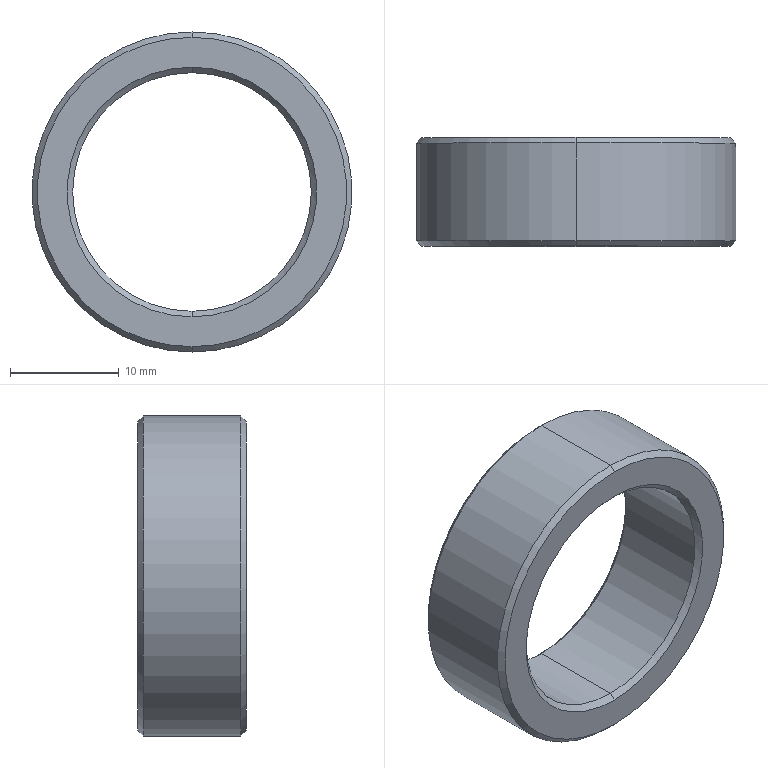Part | STEP file | Cuon T phu H01_3 | 1 solid | 14 faces | box 29.5 x 10 x 29.5 mm | volume 2993 mm3 | cone 8 | cylinder 4 | plane 2 | commonest cylinder face diameters 22 x2 29.5 x2
STEP:
#1=CARTESIAN_POINT('',(0.,0.,0.));
#2=DIRECTION('',(0.,0.,1.));
#3=DIRECTION('',(1.,0.,0.));
#4=AXIS2_PLACEMENT_3D('',#1,#2,#3);
#5=CARTESIAN_POINT('',(0.,9.5,11.));
#6=VERTEX_POINT('',#5);
#7=CARTESIAN_POINT('',(0.,10.,11.5));
#8=VERTEX_POINT('',#7);
#9=CARTESIAN_POINT('',(0.,9.5,11.));
#10=DIRECTION('',(0.,0.7071,0.7071));
#11=VECTOR('',#10,1.);
#12=LINE('',#9,#11);
#13=CARTESIAN_POINT('',(0.,9.5,0.));
#14=DIRECTION('',(0.,1.,0.));
#15=DIRECTION('',(0.,0.,1.));
#16=AXIS2_PLACEMENT_3D('',#13,#14,#15);
#17=CONICAL_SURFACE('',#16,11.,0.7854);
#18=CARTESIAN_POINT('',(6.283,0.));
#19=DIRECTION('',(0.,1.));
#20=VECTOR('',#19,1.);
#21=LINE('',#18,#20);
#22=(GEOMETRIC_REPRESENTATION_CONTEXT(2)PARAMETRIC_REPRESENTATION_CONTEXT()REPRESENTATION_CONTEXT('',''));
#23=DEFINITIONAL_REPRESENTATION('',(#21),#22);
#24=PCURVE('',#17,#23);
#25=CARTESIAN_POINT('',(0.,9.5,0.));
#26=DIRECTION('',(0.,1.,0.));
#27=DIRECTION('',(0.,0.,1.));
#28=AXIS2_PLACEMENT_3D('',#25,#26,#27);
#29=CONICAL_SURFACE('',#28,11.,0.7854);
#30=CARTESIAN_POINT('',(0.,0.));
#31=DIRECTION('',(0.,1.));
#32=VECTOR('',#31,1.);
#33=LINE('',#30,#32);
#34=(GEOMETRIC_REPRESENTATION_CONTEXT(2)PARAMETRIC_REPRESENTATION_CONTEXT()REPRESENTATION_CONTEXT('',''));
#35=DEFINITIONAL_REPRESENTATION('',(#33),#34);
#36=PCURVE('',#29,#35);
#37=SURFACE_CURVE('',#12,(#24,#36),.PCURVE_S1.);
#38=EDGE_CURVE('',#6,#8,#37,.T.);
#39=ORIENTED_EDGE('',*,*,#38,.T.);
#40=CARTESIAN_POINT('',(0.,10.,-11.5));
#41=VERTEX_POINT('',#40);
#42=CARTESIAN_POINT('',(0.,10.,0.));
#43=DIRECTION('',(0.,-1.,0.));
#44=DIRECTION('',(0.,0.,1.));
#45=AXIS2_PLACEMENT_3D('',#42,#43,#44);
#46=CIRCLE('',#45,11.5);
#47=CARTESIAN_POINT('',(6.283,0.5));
#48=DIRECTION('',(-1.,0.));
#49=VECTOR('',#48,1.);
#50=LINE('',#47,#49);
#51=(GEOMETRIC_REPRESENTATION_CONTEXT(2)PARAMETRIC_REPRESENTATION_CONTEXT()REPRESENTATION_CONTEXT('',''));
#52=DEFINITIONAL_REPRESENTATION('',(#50),#51);
#53=PCURVE('',#17,#52);
#54=CARTESIAN_POINT('',(0.,10.,0.));
#55=DIRECTION('',(0.,1.,0.));
#56=DIRECTION('',(0.,0.,1.));
#57=AXIS2_PLACEMENT_3D('',#54,#55,#56);
#58=PLANE('',#57);
#59=CARTESIAN_POINT('',(11.5,0.));
#60=CARTESIAN_POINT('',(11.5,-19.919));
#61=CARTESIAN_POINT('',(-5.75,-9.959));
#62=CARTESIAN_POINT('',(-23.,0.));
#63=CARTESIAN_POINT('',(-5.75,9.959));
#64=CARTESIAN_POINT('',(11.5,19.919));
#65=CARTESIAN_POINT('',(11.5,0.));
#66=(BOUNDED_CURVE()B_SPLINE_CURVE(2,(#59,#60,#61,#62,#63,#64,#65),.UNSPECIFIED.,.T.,.F.)B_SPLINE_CURVE_WITH_KNOTS((1,2,2,2,2,1),(-2.094,0.,2.094,4.189,6.283,8.378),.UNSPECIFIED.)CURVE()GEOMETRIC_REPRESENTATION_ITEM()RATIONAL_B_SPLINE_CURVE((1.,0.5,1.,0.5,1.,0.5,1.))REPRESENTATION_ITEM(''));
#67=(GEOMETRIC_REPRESENTATION_CONTEXT(2)PARAMETRIC_REPRESENTATION_CONTEXT()REPRESENTATION_CONTEXT('',''));
#68=DEFINITIONAL_REPRESENTATION('',(#66),#67);
#69=PCURVE('',#58,#68);
#70=SURFACE_CURVE('',#46,(#53,#69),.PCURVE_S1.);
#71=EDGE_CURVE('',#8,#41,#70,.T.);
#72=ORIENTED_EDGE('',*,*,#71,.T.);
#73=CARTESIAN_POINT('',(0.,9.5,-11.));
#74=VERTEX_POINT('',#73);
#75=CARTESIAN_POINT('',(0.,9.5,-11.));
#76=DIRECTION('',(0.,0.7071,-0.7071));
#77=VECTOR('',#76,1.);
#78=LINE('',#75,#77);
#79=CARTESIAN_POINT('',(3.142,0.));
#80=DIRECTION('',(0.,1.));
#81=VECTOR('',#80,1.);
#82=LINE('',#79,#81);
#83=(GEOMETRIC_REPRESENTATION_CONTEXT(2)PARAMETRIC_REPRESENTATION_CONTEXT()REPRESENTATION_CONTEXT('',''));
#84=DEFINITIONAL_REPRESENTATION('',(#82),#83);
#85=PCURVE('',#17,#84);
#86=CARTESIAN_POINT('',(3.142,0.));
#87=DIRECTION('',(0.,1.));
#88=VECTOR('',#87,1.);
#89=LINE('',#86,#88);
#90=(GEOMETRIC_REPRESENTATION_CONTEXT(2)PARAMETRIC_REPRESENTATION_CONTEXT()REPRESENTATION_CONTEXT('',''));
#91=DEFINITIONAL_REPRESENTATION('',(#89),#90);
#92=PCURVE('',#29,#91);
#93=SURFACE_CURVE('',#78,(#85,#92),.PCURVE_S1.);
#94=EDGE_CURVE('',#74,#41,#93,.T.);
#95=ORIENTED_EDGE('',*,*,#94,.F.);
#96=CARTESIAN_POINT('',(0.,9.5,0.));
#97=DIRECTION('',(0.,1.,0.));
#98=DIRECTION('',(0.,0.,1.));
#99=AXIS2_PLACEMENT_3D('',#96,#97,#98);
#100=CIRCLE('',#99,11.);
#101=CARTESIAN_POINT('',(0.,0.));
#102=DIRECTION('',(1.,0.));
#103=VECTOR('',#102,1.);
#104=LINE('',#101,#103);
#105=(GEOMETRIC_REPRESENTATION_CONTEXT(2)PARAMETRIC_REPRESENTATION_CONTEXT()REPRESENTATION_CONTEXT('',''));
#106=DEFINITIONAL_REPRESENTATION('',(#104),#105);
#107=PCURVE('',#17,#106);
#108=CARTESIAN_POINT('',(0.,10.,0.));
#109=DIRECTION('',(0.,-1.,0.));
#110=DIRECTION('',(0.,0.,-1.));
#111=AXIS2_PLACEMENT_3D('',#108,#109,#110);
#112=CYLINDRICAL_SURFACE('',#111,11.);
#113=CARTESIAN_POINT('',(9.425,0.5));
#114=DIRECTION('',(-1.,0.));
#115=VECTOR('',#114,1.);
#116=LINE('',#113,#115);
#117=(GEOMETRIC_REPRESENTATION_CONTEXT(2)PARAMETRIC_REPRESENTATION_CONTEXT()REPRESENTATION_CONTEXT('',''));
#118=DEFINITIONAL_REPRESENTATION('',(#116),#117);
#119=PCURVE('',#112,#118);
#120=SURFACE_CURVE('',#100,(#107,#119),.PCURVE_S1.);
#121=EDGE_CURVE('',#74,#6,#120,.T.);
#122=ORIENTED_EDGE('',*,*,#121,.T.);
#123=EDGE_LOOP('',(#39,#72,#95,#122));
#124=FACE_BOUND('',#123,.F.);
#125=ADVANCED_FACE('',(#124),#17,.F.);
#126=CARTESIAN_POINT('',(0.,0.5,-11.));
#127=VERTEX_POINT('',#126);
#128=CARTESIAN_POINT('',(0.,0.,-11.5));
#129=VERTEX_POINT('',#128);
#130=CARTESIAN_POINT('',(0.,0.,-11.5));
#131=DIRECTION('',(0.,-0.7071,-0.7071));
#132=VECTOR('',#131,1.);
#133=LINE('',#130,#132);
#134=CARTESIAN_POINT('',(0.,0.,0.));
#135=DIRECTION('',(0.,-1.,0.));
#136=DIRECTION('',(0.,0.,-1.));
#137=AXIS2_PLACEMENT_3D('',#134,#135,#136);
#138=CONICAL_SURFACE('',#137,11.5,0.7854);
#139=CARTESIAN_POINT('',(6.283,0.));
#140=DIRECTION('',(0.,1.));
#141=VECTOR('',#140,1.);
#142=LINE('',#139,#141);
#143=(GEOMETRIC_REPRESENTATION_CONTEXT(2)PARAMETRIC_REPRESENTATION_CONTEXT()REPRESENTATION_CONTEXT('',''));
#144=DEFINITIONAL_REPRESENTATION('',(#142),#143);
#145=PCURVE('',#138,#144);
#146=CARTESIAN_POINT('',(0.,0.,0.));
#147=DIRECTION('',(0.,-1.,0.));
#148=DIRECTION('',(0.,0.,-1.));
#149=AXIS2_PLACEMENT_3D('',#146,#147,#148);
#150=CONICAL_SURFACE('',#149,11.5,0.7854);
#151=CARTESIAN_POINT('',(0.,0.));
#152=DIRECTION('',(0.,1.));
#153=VECTOR('',#152,1.);
#154=LINE('',#151,#153);
#155=(GEOMETRIC_REPRESENTATION_CONTEXT(2)PARAMETRIC_REPRESENTATION_CONTEXT()REPRESENTATION_CONTEXT('',''));
#156=DEFINITIONAL_REPRESENTATION('',(#154),#155);
#157=PCURVE('',#150,#156);
#158=SURFACE_CURVE('',#133,(#145,#157),.PCURVE_S1.);
#159=EDGE_CURVE('',#127,#129,#158,.T.);
#160=ORIENTED_EDGE('',*,*,#159,.T.);
#161=CARTESIAN_POINT('',(0.,0.,11.5));
#162=VERTEX_POINT('',#161);
#163=CARTESIAN_POINT('',(0.,0.,0.));
#164=DIRECTION('',(0.,1.,0.));
#165=DIRECTION('',(0.,0.,1.));
#166=AXIS2_PLACEMENT_3D('',#163,#164,#165);
#167=CIRCLE('',#166,11.5);
#168=CARTESIAN_POINT('',(9.425,0.));
#169=DIRECTION('',(-1.,0.));
#170=VECTOR('',#169,1.);
#171=LINE('',#168,#170);
#172=(GEOMETRIC_REPRESENTATION_CONTEXT(2)PARAMETRIC_REPRESENTATION_CONTEXT()REPRESENTATION_CONTEXT('',''));
#173=DEFINITIONAL_REPRESENTATION('',(#171),#172);
#174=PCURVE('',#138,#173);
#175=CARTESIAN_POINT('',(0.,0.,0.));
#176=DIRECTION('',(0.,1.,0.));
#177=DIRECTION('',(0.,0.,1.));
#178=AXIS2_PLACEMENT_3D('',#175,#176,#177);
#179=PLANE('',#178);
#180=CARTESIAN_POINT('',(0.,0.));
#181=DIRECTION('',(1.,0.));
#182=AXIS2_PLACEMENT_2D('',#180,#181);
#183=CIRCLE('',#182,11.5);
#184=(GEOMETRIC_REPRESENTATION_CONTEXT(2)PARAMETRIC_REPRESENTATION_CONTEXT()REPRESENTATION_CONTEXT('',''));
#185=DEFINITIONAL_REPRESENTATION('',(#183),#184);
#186=PCURVE('',#179,#185);
#187=SURFACE_CURVE('',#167,(#174,#186),.PCURVE_S1.);
#188=EDGE_CURVE('',#129,#162,#187,.T.);
#189=ORIENTED_EDGE('',*,*,#188,.T.);
#190=CARTESIAN_POINT('',(0.,0.5,11.));
#191=VERTEX_POINT('',#190);
#192=CARTESIAN_POINT('',(0.,0.,11.5));
#193=DIRECTION('',(0.,-0.7071,0.7071));
#194=VECTOR('',#193,1.);
#195=LINE('',#192,#194);
#196=CARTESIAN_POINT('',(3.142,0.));
#197=DIRECTION('',(0.,1.));
#198=VECTOR('',#197,1.);
#199=LINE('',#196,#198);
#200=(GEOMETRIC_REPRESENTATION_CONTEXT(2)PARAMETRIC_REPRESENTATION_CONTEXT()REPRESENTATION_CONTEXT('',''));
#201=DEFINITIONAL_REPRESENTATION('',(#199),#200);
#202=PCURVE('',#138,#201);
#203=CARTESIAN_POINT('',(3.142,0.));
#204=DIRECTION('',(0.,1.));
#205=VECTOR('',#204,1.);
#206=LINE('',#203,#205);
#207=(GEOMETRIC_REPRESENTATION_CONTEXT(2)PARAMETRIC_REPRESENTATION_CONTEXT()REPRESENTATION_CONTEXT('',''));
#208=DEFINITIONAL_REPRESENTATION('',(#206),#207);
#209=PCURVE('',#150,#208);
#210=SURFACE_CURVE('',#195,(#202,#209),.PCURVE_S1.);
#211=EDGE_CURVE('',#191,#162,#210,.T.);
#212=ORIENTED_EDGE('',*,*,#211,.F.);
#213=CARTESIAN_POINT('',(0.,0.5,0.));
#214=DIRECTION('',(0.,-1.,0.));
#215=DIRECTION('',(0.,0.,1.));
#216=AXIS2_PLACEMENT_3D('',#213,#214,#215);
#217=CIRCLE('',#216,11.);
#218=CARTESIAN_POINT('',(3.142,-0.5));
#219=DIRECTION('',(1.,0.));
#220=VECTOR('',#219,1.);
#221=LINE('',#218,#220);
#222=(GEOMETRIC_REPRESENTATION_CONTEXT(2)PARAMETRIC_REPRESENTATION_CONTEXT()REPRESENTATION_CONTEXT('',''));
#223=DEFINITIONAL_REPRESENTATION('',(#221),#222);
#224=PCURVE('',#138,#223);
#225=CARTESIAN_POINT('',(3.142,9.5));
#226=DIRECTION('',(1.,0.));
#227=VECTOR('',#226,1.);
#228=LINE('',#225,#227);
#229=(GEOMETRIC_REPRESENTATION_CONTEXT(2)PARAMETRIC_REPRESENTATION_CONTEXT()REPRESENTATION_CONTEXT('',''));
#230=DEFINITIONAL_REPRESENTATION('',(#228),#229);
#231=PCURVE('',#112,#230);
#232=SURFACE_CURVE('',#217,(#224,#231),.PCURVE_S1.);
#233=EDGE_CURVE('',#191,#127,#232,.T.);
#234=ORIENTED_EDGE('',*,*,#233,.T.);
#235=EDGE_LOOP('',(#160,#189,#212,#234));
#236=FACE_BOUND('',#235,.F.);
#237=ADVANCED_FACE('',(#236),#138,.F.);
#238=CARTESIAN_POINT('',(0.,10.,14.25));
#239=VERTEX_POINT('',#238);
#240=CARTESIAN_POINT('',(0.,10.,-14.25));
#241=VERTEX_POINT('',#240);
#242=CARTESIAN_POINT('',(0.,10.,0.));
#243=DIRECTION('',(0.,1.,0.));
#244=DIRECTION('',(0.,0.,1.));
#245=AXIS2_PLACEMENT_3D('',#242,#243,#244);
#246=CIRCLE('',#245,14.25);
#247=CARTESIAN_POINT('',(0.,10.,0.));
#248=DIRECTION('',(0.,-1.,0.));
#249=DIRECTION('',(0.,0.,-1.));
#250=AXIS2_PLACEMENT_3D('',#247,#248,#249);
#251=CONICAL_SURFACE('',#250,14.25,0.7854);
#252=CARTESIAN_POINT('',(3.142,0.));
#253=DIRECTION('',(-1.,0.));
#254=VECTOR('',#253,1.);
#255=LINE('',#252,#254);
#256=(GEOMETRIC_REPRESENTATION_CONTEXT(2)PARAMETRIC_REPRESENTATION_CONTEXT()REPRESENTATION_CONTEXT('',''));
#257=DEFINITIONAL_REPRESENTATION('',(#255),#256);
#258=PCURVE('',#251,#257);
#259=CARTESIAN_POINT('',(0.,0.));
#260=DIRECTION('',(1.,0.));
#261=AXIS2_PLACEMENT_2D('',#259,#260);
#262=CIRCLE('',#261,14.25);
#263=(GEOMETRIC_REPRESENTATION_CONTEXT(2)PARAMETRIC_REPRESENTATION_CONTEXT()REPRESENTATION_CONTEXT('',''));
#264=DEFINITIONAL_REPRESENTATION('',(#262),#263);
#265=PCURVE('',#58,#264);
#266=SURFACE_CURVE('',#246,(#258,#265),.PCURVE_S1.);
#267=EDGE_CURVE('',#239,#241,#266,.T.);
#268=ORIENTED_EDGE('',*,*,#267,.F.);
#269=CARTESIAN_POINT('',(0.,9.5,14.75));
#270=VERTEX_POINT('',#269);
#271=CARTESIAN_POINT('',(0.,10.,14.25));
#272=DIRECTION('',(0.,-0.7071,0.7071));
#273=VECTOR('',#272,1.);
#274=LINE('',#271,#273);
#275=CARTESIAN_POINT('',(3.142,0.));
#276=DIRECTION('',(0.,1.));
#277=VECTOR('',#276,1.);
#278=LINE('',#275,#277);
#279=(GEOMETRIC_REPRESENTATION_CONTEXT(2)PARAMETRIC_REPRESENTATION_CONTEXT()REPRESENTATION_CONTEXT('',''));
#280=DEFINITIONAL_REPRESENTATION('',(#278),#279);
#281=PCURVE('',#251,#280);
#282=CARTESIAN_POINT('',(0.,10.,0.));
#283=DIRECTION('',(0.,-1.,0.));
#284=DIRECTION('',(0.,0.,-1.));
#285=AXIS2_PLACEMENT_3D('',#282,#283,#284);
#286=CONICAL_SURFACE('',#285,14.25,0.7854);
#287=CARTESIAN_POINT('',(3.142,0.));
#288=DIRECTION('',(0.,1.));
#289=VECTOR('',#288,1.);
#290=LINE('',#287,#289);
#291=(GEOMETRIC_REPRESENTATION_CONTEXT(2)PARAMETRIC_REPRESENTATION_CONTEXT()REPRESENTATION_CONTEXT('',''));
#292=DEFINITIONAL_REPRESENTATION('',(#290),#291);
#293=PCURVE('',#286,#292);
#294=SURFACE_CURVE('',#274,(#281,#293),.PCURVE_S1.);
#295=EDGE_CURVE('',#239,#270,#294,.T.);
#296=ORIENTED_EDGE('',*,*,#295,.T.);
#297=CARTESIAN_POINT('',(0.,9.5,-14.75));
#298=VERTEX_POINT('',#297);
#299=CARTESIAN_POINT('',(0.,9.5,0.));
#300=DIRECTION('',(0.,-1.,0.));
#301=DIRECTION('',(0.,0.,1.));
#302=AXIS2_PLACEMENT_3D('',#299,#300,#301);
#303=CIRCLE('',#302,14.75);
#304=CARTESIAN_POINT('',(-3.142,0.5));
#305=DIRECTION('',(1.,0.));
#306=VECTOR('',#305,1.);
#307=LINE('',#304,#306);
#308=(GEOMETRIC_REPRESENTATION_CONTEXT(2)PARAMETRIC_REPRESENTATION_CONTEXT()REPRESENTATION_CONTEXT('',''));
#309=DEFINITIONAL_REPRESENTATION('',(#307),#308);
#310=PCURVE('',#251,#309);
#311=CARTESIAN_POINT('',(0.,10.,0.));
#312=DIRECTION('',(0.,-1.,0.));
#313=DIRECTION('',(0.,0.,-1.));
#314=AXIS2_PLACEMENT_3D('',#311,#312,#313);
#315=CYLINDRICAL_SURFACE('',#314,14.75);
#316=CARTESIAN_POINT('',(-3.142,0.5));
#317=DIRECTION('',(1.,0.));
#318=VECTOR('',#317,1.);
#319=LINE('',#316,#318);
#320=(GEOMETRIC_REPRESENTATION_CONTEXT(2)PARAMETRIC_REPRESENTATION_CONTEXT()REPRESENTATION_CONTEXT('',''));
#321=DEFINITIONAL_REPRESENTATION('',(#319),#320);
#322=PCURVE('',#315,#321);
#323=SURFACE_CURVE('',#303,(#310,#322),.PCURVE_S1.);
#324=EDGE_CURVE('',#298,#270,#323,.T.);
#325=ORIENTED_EDGE('',*,*,#324,.F.);
#326=CARTESIAN_POINT('',(0.,10.,-14.25));
#327=DIRECTION('',(0.,-0.7071,-0.7071));
#328=VECTOR('',#327,1.);
#329=LINE('',#326,#328);
#330=CARTESIAN_POINT('',(0.,0.));
#331=DIRECTION('',(0.,1.));
#332=VECTOR('',#331,1.);
#333=LINE('',#330,#332);
#334=(GEOMETRIC_REPRESENTATION_CONTEXT(2)PARAMETRIC_REPRESENTATION_CONTEXT()REPRESENTATION_CONTEXT('',''));
#335=DEFINITIONAL_REPRESENTATION('',(#333),#334);
#336=PCURVE('',#251,#335);
#337=CARTESIAN_POINT('',(6.283,0.));
#338=DIRECTION('',(0.,1.));
#339=VECTOR('',#338,1.);
#340=LINE('',#337,#339);
#341=(GEOMETRIC_REPRESENTATION_CONTEXT(2)PARAMETRIC_REPRESENTATION_CONTEXT()REPRESENTATION_CONTEXT('',''));
#342=DEFINITIONAL_REPRESENTATION('',(#340),#341);
#343=PCURVE('',#286,#342);
#344=SURFACE_CURVE('',#329,(#336,#343),.PCURVE_S1.);
#345=EDGE_CURVE('',#241,#298,#344,.T.);
#346=ORIENTED_EDGE('',*,*,#345,.F.);
#347=EDGE_LOOP('',(#268,#296,#325,#346));
#348=FACE_BOUND('',#347,.T.);
#349=ADVANCED_FACE('',(#348),#251,.T.);
#350=CARTESIAN_POINT('',(0.,0.,-14.25));
#351=VERTEX_POINT('',#350);
#352=CARTESIAN_POINT('',(0.,0.,14.25));
#353=VERTEX_POINT('',#352);
#354=CARTESIAN_POINT('',(0.,0.,0.));
#355=DIRECTION('',(0.,-1.,0.));
#356=DIRECTION('',(0.,0.,1.));
#357=AXIS2_PLACEMENT_3D('',#354,#355,#356);
#358=CIRCLE('',#357,14.25);
#359=CARTESIAN_POINT('',(0.,0.5,0.));
#360=DIRECTION('',(0.,1.,0.));
#361=DIRECTION('',(0.,0.,1.));
#362=AXIS2_PLACEMENT_3D('',#359,#360,#361);
#363=CONICAL_SURFACE('',#362,14.75,0.7854);
#364=CARTESIAN_POINT('',(6.283,-0.5));
#365=DIRECTION('',(-1.,0.));
#366=VECTOR('',#365,1.);
#367=LINE('',#364,#366);
#368=(GEOMETRIC_REPRESENTATION_CONTEXT(2)PARAMETRIC_REPRESENTATION_CONTEXT()REPRESENTATION_CONTEXT('',''));
#369=DEFINITIONAL_REPRESENTATION('',(#367),#368);
#370=PCURVE('',#363,#369);
#371=CARTESIAN_POINT('',(14.25,0.));
#372=CARTESIAN_POINT('',(14.25,-24.682));
#373=CARTESIAN_POINT('',(-7.125,-12.341));
#374=CARTESIAN_POINT('',(-28.5,0.));
#375=CARTESIAN_POINT('',(-7.125,12.341));
#376=CARTESIAN_POINT('',(14.25,24.682));
#377=CARTESIAN_POINT('',(14.25,0.));
#378=(BOUNDED_CURVE()B_SPLINE_CURVE(2,(#371,#372,#373,#374,#375,#376,#377),.UNSPECIFIED.,.T.,.F.)B_SPLINE_CURVE_WITH_KNOTS((1,2,2,2,2,1),(-2.094,0.,2.094,4.189,6.283,8.378),.UNSPECIFIED.)CURVE()GEOMETRIC_REPRESENTATION_ITEM()RATIONAL_B_SPLINE_CURVE((1.,0.5,1.,0.5,1.,0.5,1.))REPRESENTATION_ITEM(''));
#379=(GEOMETRIC_REPRESENTATION_CONTEXT(2)PARAMETRIC_REPRESENTATION_CONTEXT()REPRESENTATION_CONTEXT('',''));
#380=DEFINITIONAL_REPRESENTATION('',(#378),#379);
#381=PCURVE('',#179,#380);
#382=SURFACE_CURVE('',#358,(#370,#381),.PCURVE_S1.);
#383=EDGE_CURVE('',#351,#353,#382,.T.);
#384=ORIENTED_EDGE('',*,*,#383,.F.);
#385=CARTESIAN_POINT('',(0.,0.5,-14.75));
#386=VERTEX_POINT('',#385);
#387=CARTESIAN_POINT('',(0.,0.5,-14.75));
#388=DIRECTION('',(0.,0.7071,-0.7071));
#389=VECTOR('',#388,1.);
#390=LINE('',#387,#389);
#391=CARTESIAN_POINT('',(3.142,0.));
#392=DIRECTION('',(0.,1.));
#393=VECTOR('',#392,1.);
#394=LINE('',#391,#393);
#395=(GEOMETRIC_REPRESENTATION_CONTEXT(2)PARAMETRIC_REPRESENTATION_CONTEXT()REPRESENTATION_CONTEXT('',''));
#396=DEFINITIONAL_REPRESENTATION('',(#394),#395);
#397=PCURVE('',#363,#396);
#398=CARTESIAN_POINT('',(0.,0.5,0.));
#399=DIRECTION('',(0.,1.,0.));
#400=DIRECTION('',(0.,0.,1.));
#401=AXIS2_PLACEMENT_3D('',#398,#399,#400);
#402=CONICAL_SURFACE('',#401,14.75,0.7854);
#403=CARTESIAN_POINT('',(3.142,0.));
#404=DIRECTION('',(0.,1.));
#405=VECTOR('',#404,1.);
#406=LINE('',#403,#405);
#407=(GEOMETRIC_REPRESENTATION_CONTEXT(2)PARAMETRIC_REPRESENTATION_CONTEXT()REPRESENTATION_CONTEXT('',''));
#408=DEFINITIONAL_REPRESENTATION('',(#406),#407);
#409=PCURVE('',#402,#408);
#410=SURFACE_CURVE('',#390,(#397,#409),.PCURVE_S1.);
#411=EDGE_CURVE('',#351,#386,#410,.T.);
#412=ORIENTED_EDGE('',*,*,#411,.T.);
#413=CARTESIAN_POINT('',(0.,0.5,14.75));
#414=VERTEX_POINT('',#413);
#415=CARTESIAN_POINT('',(0.,0.5,0.));
#416=DIRECTION('',(0.,1.,0.));
#417=DIRECTION('',(0.,0.,1.));
#418=AXIS2_PLACEMENT_3D('',#415,#416,#417);
#419=CIRCLE('',#418,14.75);
#420=CARTESIAN_POINT('',(0.,0.));
#421=DIRECTION('',(1.,0.));
#422=VECTOR('',#421,1.);
#423=LINE('',#420,#422);
#424=(GEOMETRIC_REPRESENTATION_CONTEXT(2)PARAMETRIC_REPRESENTATION_CONTEXT()REPRESENTATION_CONTEXT('',''));
#425=DEFINITIONAL_REPRESENTATION('',(#423),#424);
#426=PCURVE('',#363,#425);
#427=CARTESIAN_POINT('',(3.142,9.5));
#428=DIRECTION('',(-1.,0.));
#429=VECTOR('',#428,1.);
#430=LINE('',#427,#429);
#431=(GEOMETRIC_REPRESENTATION_CONTEXT(2)PARAMETRIC_REPRESENTATION_CONTEXT()REPRESENTATION_CONTEXT('',''));
#432=DEFINITIONAL_REPRESENTATION('',(#430),#431);
#433=PCURVE('',#315,#432);
#434=SURFACE_CURVE('',#419,(#426,#433),.PCURVE_S1.);
#435=EDGE_CURVE('',#414,#386,#434,.T.);
#436=ORIENTED_EDGE('',*,*,#435,.F.);
#437=CARTESIAN_POINT('',(0.,0.5,14.75));
#438=DIRECTION('',(0.,0.7071,0.7071));
#439=VECTOR('',#438,1.);
#440=LINE('',#437,#439);
#441=CARTESIAN_POINT('',(0.,0.));
#442=DIRECTION('',(0.,1.));
#443=VECTOR('',#442,1.);
#444=LINE('',#441,#443);
#445=(GEOMETRIC_REPRESENTATION_CONTEXT(2)PARAMETRIC_REPRESENTATION_CONTEXT()REPRESENTATION_CONTEXT('',''));
#446=DEFINITIONAL_REPRESENTATION('',(#444),#445);
#447=PCURVE('',#363,#446);
#448=CARTESIAN_POINT('',(6.283,0.));
#449=DIRECTION('',(0.,1.));
#450=VECTOR('',#449,1.);
#451=LINE('',#448,#450);
#452=(GEOMETRIC_REPRESENTATION_CONTEXT(2)PARAMETRIC_REPRESENTATION_CONTEXT()REPRESENTATION_CONTEXT('',''));
#453=DEFINITIONAL_REPRESENTATION('',(#451),#452);
#454=PCURVE('',#402,#453);
#455=SURFACE_CURVE('',#440,(#447,#454),.PCURVE_S1.);
#456=EDGE_CURVE('',#353,#414,#455,.T.);
#457=ORIENTED_EDGE('',*,*,#456,.F.);
#458=EDGE_LOOP('',(#384,#412,#436,#457));
#459=FACE_BOUND('',#458,.T.);
#460=ADVANCED_FACE('',(#459),#363,.T.);
#461=CARTESIAN_POINT('',(0.,10.,-11.));
#462=DIRECTION('',(0.,-1.,0.));
#463=VECTOR('',#462,1.);
#464=LINE('',#461,#463);
#465=CARTESIAN_POINT('',(6.283,0.));
#466=DIRECTION('',(0.,1.));
#467=VECTOR('',#466,1.);
#468=LINE('',#465,#467);
#469=(GEOMETRIC_REPRESENTATION_CONTEXT(2)PARAMETRIC_REPRESENTATION_CONTEXT()REPRESENTATION_CONTEXT('',''));
#470=DEFINITIONAL_REPRESENTATION('',(#468),#469);
#471=PCURVE('',#112,#470);
#472=CARTESIAN_POINT('',(0.,10.,0.));
#473=DIRECTION('',(0.,-1.,0.));
#474=DIRECTION('',(0.,0.,-1.));
#475=AXIS2_PLACEMENT_3D('',#472,#473,#474);
#476=CYLINDRICAL_SURFACE('',#475,11.);
#477=CARTESIAN_POINT('',(0.,0.));
#478=DIRECTION('',(0.,1.));
#479=VECTOR('',#478,1.);
#480=LINE('',#477,#479);
#481=(GEOMETRIC_REPRESENTATION_CONTEXT(2)PARAMETRIC_REPRESENTATION_CONTEXT()REPRESENTATION_CONTEXT('',''));
#482=DEFINITIONAL_REPRESENTATION('',(#480),#481);
#483=PCURVE('',#476,#482);
#484=SURFACE_CURVE('',#464,(#471,#483),.PCURVE_S1.);
#485=EDGE_CURVE('',#74,#127,#484,.T.);
#486=ORIENTED_EDGE('',*,*,#485,.T.);
#487=ORIENTED_EDGE('',*,*,#233,.F.);
#488=CARTESIAN_POINT('',(0.,10.,11.));
#489=DIRECTION('',(0.,-1.,0.));
#490=VECTOR('',#489,1.);
#491=LINE('',#488,#490);
#492=CARTESIAN_POINT('',(3.142,0.));
#493=DIRECTION('',(0.,1.));
#494=VECTOR('',#493,1.);
#495=LINE('',#492,#494);
#496=(GEOMETRIC_REPRESENTATION_CONTEXT(2)PARAMETRIC_REPRESENTATION_CONTEXT()REPRESENTATION_CONTEXT('',''));
#497=DEFINITIONAL_REPRESENTATION('',(#495),#496);
#498=PCURVE('',#112,#497);
#499=CARTESIAN_POINT('',(3.142,0.));
#500=DIRECTION('',(0.,1.));
#501=VECTOR('',#500,1.);
#502=LINE('',#499,#501);
#503=(GEOMETRIC_REPRESENTATION_CONTEXT(2)PARAMETRIC_REPRESENTATION_CONTEXT()REPRESENTATION_CONTEXT('',''));
#504=DEFINITIONAL_REPRESENTATION('',(#502),#503);
#505=PCURVE('',#476,#504);
#506=SURFACE_CURVE('',#491,(#498,#505),.PCURVE_S1.);
#507=EDGE_CURVE('',#6,#191,#506,.T.);
#508=ORIENTED_EDGE('',*,*,#507,.F.);
#509=ORIENTED_EDGE('',*,*,#121,.F.);
#510=EDGE_LOOP('',(#486,#487,#508,#509));
#511=FACE_BOUND('',#510,.F.);
#512=ADVANCED_FACE('',(#511),#112,.F.);
#513=ORIENTED_EDGE('',*,*,#324,.T.);
#514=CARTESIAN_POINT('',(0.,10.,14.75));
#515=DIRECTION('',(0.,-1.,0.));
#516=VECTOR('',#515,1.);
#517=LINE('',#514,#516);
#518=CARTESIAN_POINT('',(3.142,0.));
#519=DIRECTION('',(0.,1.));
#520=VECTOR('',#519,1.);
#521=LINE('',#518,#520);
#522=(GEOMETRIC_REPRESENTATION_CONTEXT(2)PARAMETRIC_REPRESENTATION_CONTEXT()REPRESENTATION_CONTEXT('',''));
#523=DEFINITIONAL_REPRESENTATION('',(#521),#522);
#524=PCURVE('',#315,#523);
#525=CARTESIAN_POINT('',(0.,10.,0.));
#526=DIRECTION('',(0.,-1.,0.));
#527=DIRECTION('',(0.,0.,-1.));
#528=AXIS2_PLACEMENT_3D('',#525,#526,#527);
#529=CYLINDRICAL_SURFACE('',#528,14.75);
#530=CARTESIAN_POINT('',(3.142,0.));
#531=DIRECTION('',(0.,1.));
#532=VECTOR('',#531,1.);
#533=LINE('',#530,#532);
#534=(GEOMETRIC_REPRESENTATION_CONTEXT(2)PARAMETRIC_REPRESENTATION_CONTEXT()REPRESENTATION_CONTEXT('',''));
#535=DEFINITIONAL_REPRESENTATION('',(#533),#534);
#536=PCURVE('',#529,#535);
#537=SURFACE_CURVE('',#517,(#524,#536),.PCURVE_S1.);
#538=EDGE_CURVE('',#270,#414,#537,.T.);
#539=ORIENTED_EDGE('',*,*,#538,.T.);
#540=ORIENTED_EDGE('',*,*,#435,.T.);
#541=CARTESIAN_POINT('',(0.,10.,-14.75));
#542=DIRECTION('',(0.,-1.,0.));
#543=VECTOR('',#542,1.);
#544=LINE('',#541,#543);
#545=CARTESIAN_POINT('',(0.,0.));
#546=DIRECTION('',(0.,1.));
#547=VECTOR('',#546,1.);
#548=LINE('',#545,#547);
#549=(GEOMETRIC_REPRESENTATION_CONTEXT(2)PARAMETRIC_REPRESENTATION_CONTEXT()REPRESENTATION_CONTEXT('',''));
#550=DEFINITIONAL_REPRESENTATION('',(#548),#549);
#551=PCURVE('',#315,#550);
#552=CARTESIAN_POINT('',(6.283,0.));
#553=DIRECTION('',(0.,1.));
#554=VECTOR('',#553,1.);
#555=LINE('',#552,#554);
#556=(GEOMETRIC_REPRESENTATION_CONTEXT(2)PARAMETRIC_REPRESENTATION_CONTEXT()REPRESENTATION_CONTEXT('',''));
#557=DEFINITIONAL_REPRESENTATION('',(#555),#556);
#558=PCURVE('',#529,#557);
#559=SURFACE_CURVE('',#544,(#551,#558),.PCURVE_S1.);
#560=EDGE_CURVE('',#298,#386,#559,.T.);
#561=ORIENTED_EDGE('',*,*,#560,.F.);
#562=EDGE_LOOP('',(#513,#539,#540,#561));
#563=FACE_BOUND('',#562,.T.);
#564=ADVANCED_FACE('',(#563),#315,.T.);
#565=CARTESIAN_POINT('',(0.,10.,0.));
#566=DIRECTION('',(0.,1.,0.));
#567=DIRECTION('',(0.,0.,1.));
#568=AXIS2_PLACEMENT_3D('',#565,#566,#567);
#569=CIRCLE('',#568,14.25);
#570=CARTESIAN_POINT('',(0.,0.));
#571=DIRECTION('',(1.,0.));
#572=AXIS2_PLACEMENT_2D('',#570,#571);
#573=CIRCLE('',#572,14.25);
#574=(GEOMETRIC_REPRESENTATION_CONTEXT(2)PARAMETRIC_REPRESENTATION_CONTEXT()REPRESENTATION_CONTEXT('',''));
#575=DEFINITIONAL_REPRESENTATION('',(#573),#574);
#576=PCURVE('',#58,#575);
#577=CARTESIAN_POINT('',(9.425,0.));
#578=DIRECTION('',(-1.,0.));
#579=VECTOR('',#578,1.);
#580=LINE('',#577,#579);
#581=(GEOMETRIC_REPRESENTATION_CONTEXT(2)PARAMETRIC_REPRESENTATION_CONTEXT()REPRESENTATION_CONTEXT('',''));
#582=DEFINITIONAL_REPRESENTATION('',(#580),#581);
#583=PCURVE('',#286,#582);
#584=SURFACE_CURVE('',#569,(#576,#583),.PCURVE_S1.);
#585=EDGE_CURVE('',#241,#239,#584,.T.);
#586=ORIENTED_EDGE('',*,*,#585,.T.);
#587=ORIENTED_EDGE('',*,*,#267,.T.);
#588=EDGE_LOOP('',(#586,#587));
#589=FACE_BOUND('',#588,.T.);
#590=ORIENTED_EDGE('',*,*,#71,.T.);
#591=CARTESIAN_POINT('',(0.,10.,0.));
#592=DIRECTION('',(0.,-1.,0.));
#593=DIRECTION('',(0.,0.,1.));
#594=AXIS2_PLACEMENT_3D('',#591,#592,#593);
#595=CIRCLE('',#594,11.5);
#596=CARTESIAN_POINT('',(11.5,0.));
#597=CARTESIAN_POINT('',(11.5,-19.919));
#598=CARTESIAN_POINT('',(-5.75,-9.959));
#599=CARTESIAN_POINT('',(-23.,0.));
#600=CARTESIAN_POINT('',(-5.75,9.959));
#601=CARTESIAN_POINT('',(11.5,19.919));
#602=CARTESIAN_POINT('',(11.5,0.));
#603=(BOUNDED_CURVE()B_SPLINE_CURVE(2,(#596,#597,#598,#599,#600,#601,#602),.UNSPECIFIED.,.T.,.F.)B_SPLINE_CURVE_WITH_KNOTS((1,2,2,2,2,1),(-2.094,0.,2.094,4.189,6.283,8.378),.UNSPECIFIED.)CURVE()GEOMETRIC_REPRESENTATION_ITEM()RATIONAL_B_SPLINE_CURVE((1.,0.5,1.,0.5,1.,0.5,1.))REPRESENTATION_ITEM(''));
#604=(GEOMETRIC_REPRESENTATION_CONTEXT(2)PARAMETRIC_REPRESENTATION_CONTEXT()REPRESENTATION_CONTEXT('',''));
#605=DEFINITIONAL_REPRESENTATION('',(#603),#604);
#606=PCURVE('',#58,#605);
#607=CARTESIAN_POINT('',(6.283,0.5));
#608=DIRECTION('',(-1.,0.));
#609=VECTOR('',#608,1.);
#610=LINE('',#607,#609);
#611=(GEOMETRIC_REPRESENTATION_CONTEXT(2)PARAMETRIC_REPRESENTATION_CONTEXT()REPRESENTATION_CONTEXT('',''));
#612=DEFINITIONAL_REPRESENTATION('',(#610),#611);
#613=PCURVE('',#29,#612);
#614=SURFACE_CURVE('',#595,(#606,#613),.PCURVE_S1.);
#615=EDGE_CURVE('',#41,#8,#614,.T.);
#616=ORIENTED_EDGE('',*,*,#615,.T.);
#617=EDGE_LOOP('',(#590,#616));
#618=FACE_BOUND('',#617,.T.);
#619=ADVANCED_FACE('',(#589,#618),#58,.T.);
#620=CARTESIAN_POINT('',(0.,0.,0.));
#621=DIRECTION('',(0.,-1.,0.));
#622=DIRECTION('',(0.,0.,1.));
#623=AXIS2_PLACEMENT_3D('',#620,#621,#622);
#624=CIRCLE('',#623,14.25);
#625=CARTESIAN_POINT('',(14.25,0.));
#626=CARTESIAN_POINT('',(14.25,-24.682));
#627=CARTESIAN_POINT('',(-7.125,-12.341));
#628=CARTESIAN_POINT('',(-28.5,0.));
#629=CARTESIAN_POINT('',(-7.125,12.341));
#630=CARTESIAN_POINT('',(14.25,24.682));
#631=CARTESIAN_POINT('',(14.25,0.));
#632=(BOUNDED_CURVE()B_SPLINE_CURVE(2,(#625,#626,#627,#628,#629,#630,#631),.UNSPECIFIED.,.T.,.F.)B_SPLINE_CURVE_WITH_KNOTS((1,2,2,2,2,1),(-2.094,0.,2.094,4.189,6.283,8.378),.UNSPECIFIED.)CURVE()GEOMETRIC_REPRESENTATION_ITEM()RATIONAL_B_SPLINE_CURVE((1.,0.5,1.,0.5,1.,0.5,1.))REPRESENTATION_ITEM(''));
#633=(GEOMETRIC_REPRESENTATION_CONTEXT(2)PARAMETRIC_REPRESENTATION_CONTEXT()REPRESENTATION_CONTEXT('',''));
#634=DEFINITIONAL_REPRESENTATION('',(#632),#633);
#635=PCURVE('',#179,#634);
#636=CARTESIAN_POINT('',(6.283,-0.5));
#637=DIRECTION('',(-1.,0.));
#638=VECTOR('',#637,1.);
#639=LINE('',#636,#638);
#640=(GEOMETRIC_REPRESENTATION_CONTEXT(2)PARAMETRIC_REPRESENTATION_CONTEXT()REPRESENTATION_CONTEXT('',''));
#641=DEFINITIONAL_REPRESENTATION('',(#639),#640);
#642=PCURVE('',#402,#641);
#643=SURFACE_CURVE('',#624,(#635,#642),.PCURVE_S1.);
#644=EDGE_CURVE('',#353,#351,#643,.T.);
#645=ORIENTED_EDGE('',*,*,#644,.T.);
#646=ORIENTED_EDGE('',*,*,#383,.T.);
#647=EDGE_LOOP('',(#645,#646));
#648=FACE_BOUND('',#647,.T.);
#649=ORIENTED_EDGE('',*,*,#188,.T.);
#650=CARTESIAN_POINT('',(0.,0.,0.));
#651=DIRECTION('',(0.,1.,0.));
#652=DIRECTION('',(0.,0.,1.));
#653=AXIS2_PLACEMENT_3D('',#650,#651,#652);
#654=CIRCLE('',#653,11.5);
#655=CARTESIAN_POINT('',(0.,0.));
#656=DIRECTION('',(1.,0.));
#657=AXIS2_PLACEMENT_2D('',#655,#656);
#658=CIRCLE('',#657,11.5);
#659=(GEOMETRIC_REPRESENTATION_CONTEXT(2)PARAMETRIC_REPRESENTATION_CONTEXT()REPRESENTATION_CONTEXT('',''));
#660=DEFINITIONAL_REPRESENTATION('',(#658),#659);
#661=PCURVE('',#179,#660);
#662=CARTESIAN_POINT('',(3.142,0.));
#663=DIRECTION('',(-1.,0.));
#664=VECTOR('',#663,1.);
#665=LINE('',#662,#664);
#666=(GEOMETRIC_REPRESENTATION_CONTEXT(2)PARAMETRIC_REPRESENTATION_CONTEXT()REPRESENTATION_CONTEXT('',''));
#667=DEFINITIONAL_REPRESENTATION('',(#665),#666);
#668=PCURVE('',#150,#667);
#669=SURFACE_CURVE('',#654,(#661,#668),.PCURVE_S1.);
#670=EDGE_CURVE('',#162,#129,#669,.T.);
#671=ORIENTED_EDGE('',*,*,#670,.T.);
#672=EDGE_LOOP('',(#649,#671));
#673=FACE_BOUND('',#672,.T.);
#674=ADVANCED_FACE('',(#648,#673),#179,.F.);
#675=ORIENTED_EDGE('',*,*,#538,.F.);
#676=CARTESIAN_POINT('',(0.,9.5,0.));
#677=DIRECTION('',(0.,-1.,0.));
#678=DIRECTION('',(0.,0.,1.));
#679=AXIS2_PLACEMENT_3D('',#676,#677,#678);
#680=CIRCLE('',#679,14.75);
#681=CARTESIAN_POINT('',(3.142,0.5));
#682=DIRECTION('',(1.,0.));
#683=VECTOR('',#682,1.);
#684=LINE('',#681,#683);
#685=(GEOMETRIC_REPRESENTATION_CONTEXT(2)PARAMETRIC_REPRESENTATION_CONTEXT()REPRESENTATION_CONTEXT('',''));
#686=DEFINITIONAL_REPRESENTATION('',(#684),#685);
#687=PCURVE('',#529,#686);
#688=CARTESIAN_POINT('',(3.142,0.5));
#689=DIRECTION('',(1.,0.));
#690=VECTOR('',#689,1.);
#691=LINE('',#688,#690);
#692=(GEOMETRIC_REPRESENTATION_CONTEXT(2)PARAMETRIC_REPRESENTATION_CONTEXT()REPRESENTATION_CONTEXT('',''));
#693=DEFINITIONAL_REPRESENTATION('',(#691),#692);
#694=PCURVE('',#286,#693);
#695=SURFACE_CURVE('',#680,(#687,#694),.PCURVE_S1.);
#696=EDGE_CURVE('',#270,#298,#695,.T.);
#697=ORIENTED_EDGE('',*,*,#696,.T.);
#698=ORIENTED_EDGE('',*,*,#560,.T.);
#699=CARTESIAN_POINT('',(0.,0.5,0.));
#700=DIRECTION('',(0.,1.,0.));
#701=DIRECTION('',(0.,0.,1.));
#702=AXIS2_PLACEMENT_3D('',#699,#700,#701);
#703=CIRCLE('',#702,14.75);
#704=CARTESIAN_POINT('',(9.425,9.5));
#705=DIRECTION('',(-1.,0.));
#706=VECTOR('',#705,1.);
#707=LINE('',#704,#706);
#708=(GEOMETRIC_REPRESENTATION_CONTEXT(2)PARAMETRIC_REPRESENTATION_CONTEXT()REPRESENTATION_CONTEXT('',''));
#709=DEFINITIONAL_REPRESENTATION('',(#707),#708);
#710=PCURVE('',#529,#709);
#711=CARTESIAN_POINT('',(0.,0.));
#712=DIRECTION('',(1.,0.));
#713=VECTOR('',#712,1.);
#714=LINE('',#711,#713);
#715=(GEOMETRIC_REPRESENTATION_CONTEXT(2)PARAMETRIC_REPRESENTATION_CONTEXT()REPRESENTATION_CONTEXT('',''));
#716=DEFINITIONAL_REPRESENTATION('',(#714),#715);
#717=PCURVE('',#402,#716);
#718=SURFACE_CURVE('',#703,(#710,#717),.PCURVE_S1.);
#719=EDGE_CURVE('',#386,#414,#718,.T.);
#720=ORIENTED_EDGE('',*,*,#719,.T.);
#721=EDGE_LOOP('',(#675,#697,#698,#720));
#722=FACE_BOUND('',#721,.T.);
#723=ADVANCED_FACE('',(#722),#529,.T.);
#724=CARTESIAN_POINT('',(0.,0.5,0.));
#725=DIRECTION('',(0.,-1.,0.));
#726=DIRECTION('',(0.,0.,1.));
#727=AXIS2_PLACEMENT_3D('',#724,#725,#726);
#728=CIRCLE('',#727,11.);
#729=CARTESIAN_POINT('',(-3.142,9.5));
#730=DIRECTION('',(1.,0.));
#731=VECTOR('',#730,1.);
#732=LINE('',#729,#731);
#733=(GEOMETRIC_REPRESENTATION_CONTEXT(2)PARAMETRIC_REPRESENTATION_CONTEXT()REPRESENTATION_CONTEXT('',''));
#734=DEFINITIONAL_REPRESENTATION('',(#732),#733);
#735=PCURVE('',#476,#734);
#736=CARTESIAN_POINT('',(-3.142,-0.5));
#737=DIRECTION('',(1.,0.));
#738=VECTOR('',#737,1.);
#739=LINE('',#736,#738);
#740=(GEOMETRIC_REPRESENTATION_CONTEXT(2)PARAMETRIC_REPRESENTATION_CONTEXT()REPRESENTATION_CONTEXT('',''));
#741=DEFINITIONAL_REPRESENTATION('',(#739),#740);
#742=PCURVE('',#150,#741);
#743=SURFACE_CURVE('',#728,(#735,#742),.PCURVE_S1.);
#744=EDGE_CURVE('',#127,#191,#743,.T.);
#745=ORIENTED_EDGE('',*,*,#744,.F.);
#746=ORIENTED_EDGE('',*,*,#485,.F.);
#747=CARTESIAN_POINT('',(0.,9.5,0.));
#748=DIRECTION('',(0.,1.,0.));
#749=DIRECTION('',(0.,0.,1.));
#750=AXIS2_PLACEMENT_3D('',#747,#748,#749);
#751=CIRCLE('',#750,11.);
#752=CARTESIAN_POINT('',(3.142,0.5));
#753=DIRECTION('',(-1.,0.));
#754=VECTOR('',#753,1.);
#755=LINE('',#752,#754);
#756=(GEOMETRIC_REPRESENTATION_CONTEXT(2)PARAMETRIC_REPRESENTATION_CONTEXT()REPRESENTATION_CONTEXT('',''));
#757=DEFINITIONAL_REPRESENTATION('',(#755),#756);
#758=PCURVE('',#476,#757);
#759=CARTESIAN_POINT('',(0.,0.));
#760=DIRECTION('',(1.,0.));
#761=VECTOR('',#760,1.);
#762=LINE('',#759,#761);
#763=(GEOMETRIC_REPRESENTATION_CONTEXT(2)PARAMETRIC_REPRESENTATION_CONTEXT()REPRESENTATION_CONTEXT('',''));
#764=DEFINITIONAL_REPRESENTATION('',(#762),#763);
#765=PCURVE('',#29,#764);
#766=SURFACE_CURVE('',#751,(#758,#765),.PCURVE_S1.);
#767=EDGE_CURVE('',#6,#74,#766,.T.);
#768=ORIENTED_EDGE('',*,*,#767,.F.);
#769=ORIENTED_EDGE('',*,*,#507,.T.);
#770=EDGE_LOOP('',(#745,#746,#768,#769));
#771=FACE_BOUND('',#770,.F.);
#772=ADVANCED_FACE('',(#771),#476,.F.);
#773=ORIENTED_EDGE('',*,*,#411,.F.);
#774=ORIENTED_EDGE('',*,*,#644,.F.);
#775=ORIENTED_EDGE('',*,*,#456,.T.);
#776=ORIENTED_EDGE('',*,*,#719,.F.);
#777=EDGE_LOOP('',(#773,#774,#775,#776));
#778=FACE_BOUND('',#777,.T.);
#779=ADVANCED_FACE('',(#778),#402,.T.);
#780=ORIENTED_EDGE('',*,*,#295,.F.);
#781=ORIENTED_EDGE('',*,*,#585,.F.);
#782=ORIENTED_EDGE('',*,*,#345,.T.);
#783=ORIENTED_EDGE('',*,*,#696,.F.);
#784=EDGE_LOOP('',(#780,#781,#782,#783));
#785=FACE_BOUND('',#784,.T.);
#786=ADVANCED_FACE('',(#785),#286,.T.);
#787=ORIENTED_EDGE('',*,*,#670,.T.);
#788=ORIENTED_EDGE('',*,*,#159,.F.);
#789=ORIENTED_EDGE('',*,*,#744,.T.);
#790=ORIENTED_EDGE('',*,*,#211,.T.);
#791=EDGE_LOOP('',(#787,#788,#789,#790));
#792=FACE_BOUND('',#791,.F.);
#793=ADVANCED_FACE('',(#792),#150,.F.);
#794=ORIENTED_EDGE('',*,*,#615,.T.);
#795=ORIENTED_EDGE('',*,*,#38,.F.);
#796=ORIENTED_EDGE('',*,*,#767,.T.);
#797=ORIENTED_EDGE('',*,*,#94,.T.);
#798=EDGE_LOOP('',(#794,#795,#796,#797));
#799=FACE_BOUND('',#798,.F.);
#800=ADVANCED_FACE('',(#799),#29,.F.);
#801=CLOSED_SHELL('',(#125,#237,#349,#460,#512,#564,#619,#674,#723,#772,#779,#786,#793,#800));
#802=MANIFOLD_SOLID_BREP('',#801);
#803=(LENGTH_UNIT()NAMED_UNIT(*)SI_UNIT(.MILLI.,.METRE.));
#804=UNCERTAINTY_MEASURE_WITH_UNIT(LENGTH_MEASURE(0.0000001),#803,'','');
#805=(NAMED_UNIT(*)PLANE_ANGLE_UNIT()SI_UNIT($,.RADIAN.));
#806=(NAMED_UNIT(*)SI_UNIT($,.STERADIAN.)SOLID_ANGLE_UNIT());
#807=(GEOMETRIC_REPRESENTATION_CONTEXT(3)GLOBAL_UNCERTAINTY_ASSIGNED_CONTEXT((#804))GLOBAL_UNIT_ASSIGNED_CONTEXT((#803,#805,#806))REPRESENTATION_CONTEXT('',''));
#808=ADVANCED_BREP_SHAPE_REPRESENTATION('',(#4,#802),#807);